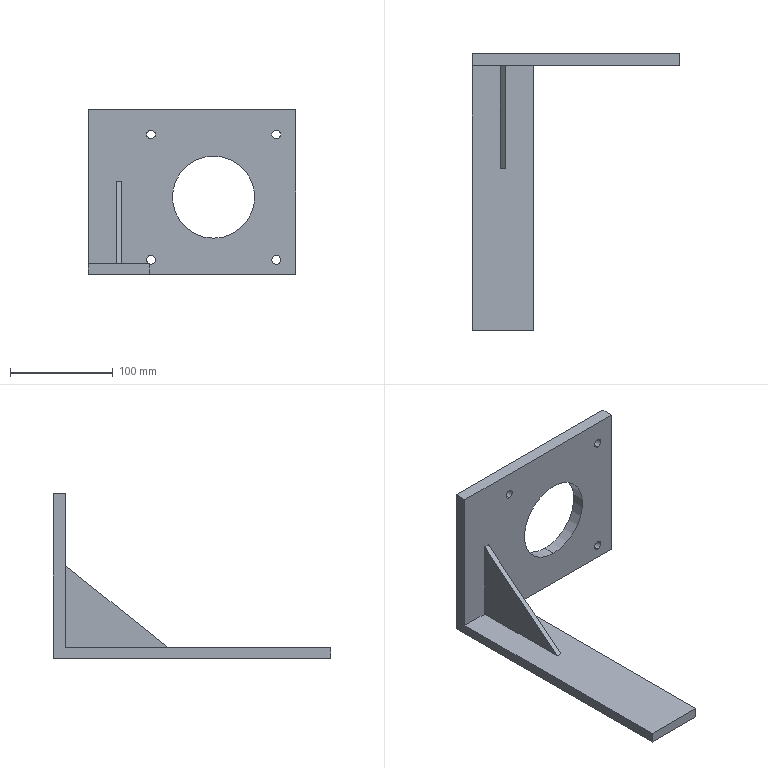Part | SolidWorks | features ICE 2, Extrusion 1, Gusset 1, HoleWzd 1 | 2 solids | 25 faces | box 202 x 270 x 160 mm | volume 499598 mm3 | plane 14 | cylinder 10 | cone 1 | commonest cylinder face diameters 8.5 x8 80 x2
STEP:
#1=CARTESIAN_POINT('',(30.,123.,9.869));
#2=VERTEX_POINT('',#1);
#3=CARTESIAN_POINT('',(31.,123.,9.75));
#4=VERTEX_POINT('',#3);
#5=CARTESIAN_POINT('',(31.,123.,14.));
#6=DIRECTION('',(0.,-1.,0.));
#7=DIRECTION('',(0.,0.,-1.));
#8=AXIS2_PLACEMENT_3D('',#5,#6,#7);
#9=CIRCLE('',#8,4.25);
#10=EDGE_CURVE('',#2,#4,#9,.T.);
#11=ORIENTED_EDGE('',*,*,#10,.T.);
#12=CARTESIAN_POINT('',(31.,135.,9.75));
#13=VERTEX_POINT('',#12);
#14=CARTESIAN_POINT('',(31.,135.,9.75));
#15=DIRECTION('',(0.,1.,0.));
#16=VECTOR('',#15,1000.);
#17=LINE('',#14,#16);
#18=EDGE_CURVE('',#4,#13,#17,.T.);
#19=ORIENTED_EDGE('',*,*,#18,.T.);
#20=CARTESIAN_POINT('',(31.,135.,18.25));
#21=VERTEX_POINT('',#20);
#22=CARTESIAN_POINT('',(31.,135.,14.));
#23=DIRECTION('',(0.,1.,0.));
#24=DIRECTION('',(0.,0.,1.));
#25=AXIS2_PLACEMENT_3D('',#22,#23,#24);
#26=CIRCLE('',#25,4.25);
#27=EDGE_CURVE('',#13,#21,#26,.T.);
#28=ORIENTED_EDGE('',*,*,#27,.T.);
#29=CARTESIAN_POINT('',(31.,123.,18.25));
#30=VERTEX_POINT('',#29);
#31=CARTESIAN_POINT('',(31.,135.,18.25));
#32=DIRECTION('',(0.,1.,0.));
#33=VECTOR('',#32,1000.);
#34=LINE('',#31,#33);
#35=EDGE_CURVE('',#30,#21,#34,.T.);
#36=ORIENTED_EDGE('',*,*,#35,.F.);
#37=CARTESIAN_POINT('',(29.564,123.,10.));
#38=VERTEX_POINT('',#37);
#39=CARTESIAN_POINT('',(31.,123.,14.));
#40=DIRECTION('',(0.,-1.,0.));
#41=DIRECTION('',(0.,0.,-1.));
#42=AXIS2_PLACEMENT_3D('',#39,#40,#41);
#43=CIRCLE('',#42,4.25);
#44=EDGE_CURVE('',#30,#38,#43,.T.);
#45=ORIENTED_EDGE('',*,*,#44,.T.);
#46=CARTESIAN_POINT('',(29.564,122.5,10.));
#47=VERTEX_POINT('',#46);
#48=CARTESIAN_POINT('',(29.564,135.,10.));
#49=DIRECTION('',(0.,1.,0.));
#50=VECTOR('',#49,1000.);
#51=LINE('',#48,#50);
#52=EDGE_CURVE('',#47,#38,#51,.T.);
#53=ORIENTED_EDGE('',*,*,#52,.F.);
#54=CARTESIAN_POINT('',(30.,122.5,9.869));
#55=VERTEX_POINT('',#54);
#56=CARTESIAN_POINT('',(31.,122.5,14.));
#57=DIRECTION('',(0.,1.,0.));
#58=DIRECTION('',(0.,0.,1.));
#59=AXIS2_PLACEMENT_3D('',#56,#57,#58);
#60=CIRCLE('',#59,4.25);
#61=EDGE_CURVE('',#55,#47,#60,.T.);
#62=ORIENTED_EDGE('',*,*,#61,.F.);
#63=CARTESIAN_POINT('',(30.,135.,9.869));
#64=DIRECTION('',(0.,-1.,0.));
#65=VECTOR('',#64,1000.);
#66=LINE('',#63,#65);
#67=EDGE_CURVE('',#2,#55,#66,.T.);
#68=ORIENTED_EDGE('',*,*,#67,.F.);
#69=EDGE_LOOP('',(#11,#19,#28,#36,#45,#53,#62,#68));
#70=FACE_OUTER_BOUND('',#69,.T.);
#71=CARTESIAN_POINT('',(31.,135.,14.));
#72=DIRECTION('',(0.,1.,0.));
#73=DIRECTION('',(0.,0.,1.));
#74=AXIS2_PLACEMENT_3D('',#71,#72,#73);
#75=CYLINDRICAL_SURFACE('',#74,4.25);
#76=ADVANCED_FACE('',(#70),#75,.F.);
#77=CARTESIAN_POINT('',(153.,123.,18.25));
#78=VERTEX_POINT('',#77);
#79=CARTESIAN_POINT('',(153.,123.,9.75));
#80=VERTEX_POINT('',#79);
#81=CARTESIAN_POINT('',(153.,123.,14.));
#82=DIRECTION('',(0.,-1.,0.));
#83=DIRECTION('',(0.,0.,-1.));
#84=AXIS2_PLACEMENT_3D('',#81,#82,#83);
#85=CIRCLE('',#84,4.25);
#86=EDGE_CURVE('',#78,#80,#85,.T.);
#87=ORIENTED_EDGE('',*,*,#86,.T.);
#88=CARTESIAN_POINT('',(153.,135.,9.75));
#89=VERTEX_POINT('',#88);
#90=CARTESIAN_POINT('',(153.,135.,9.75));
#91=DIRECTION('',(0.,1.,0.));
#92=VECTOR('',#91,1000.);
#93=LINE('',#90,#92);
#94=EDGE_CURVE('',#80,#89,#93,.T.);
#95=ORIENTED_EDGE('',*,*,#94,.T.);
#96=CARTESIAN_POINT('',(153.,135.,18.25));
#97=VERTEX_POINT('',#96);
#98=CARTESIAN_POINT('',(153.,135.,14.));
#99=DIRECTION('',(0.,1.,0.));
#100=DIRECTION('',(0.,0.,1.));
#101=AXIS2_PLACEMENT_3D('',#98,#99,#100);
#102=CIRCLE('',#101,4.25);
#103=EDGE_CURVE('',#89,#97,#102,.T.);
#104=ORIENTED_EDGE('',*,*,#103,.T.);
#105=CARTESIAN_POINT('',(153.,135.,18.25));
#106=DIRECTION('',(0.,1.,0.));
#107=VECTOR('',#106,1000.);
#108=LINE('',#105,#107);
#109=EDGE_CURVE('',#78,#97,#108,.T.);
#110=ORIENTED_EDGE('',*,*,#109,.F.);
#111=EDGE_LOOP('',(#87,#95,#104,#110));
#112=FACE_OUTER_BOUND('',#111,.T.);
#113=CARTESIAN_POINT('',(153.,135.,14.));
#114=DIRECTION('',(0.,1.,0.));
#115=DIRECTION('',(0.,0.,1.));
#116=AXIS2_PLACEMENT_3D('',#113,#114,#115);
#117=CYLINDRICAL_SURFACE('',#116,4.25);
#118=ADVANCED_FACE('',(#112),#117,.F.);
#119=CARTESIAN_POINT('',(153.,123.,140.25));
#120=VERTEX_POINT('',#119);
#121=CARTESIAN_POINT('',(153.,123.,131.75));
#122=VERTEX_POINT('',#121);
#123=CARTESIAN_POINT('',(153.,123.,136.));
#124=DIRECTION('',(0.,-1.,0.));
#125=DIRECTION('',(0.,0.,-1.));
#126=AXIS2_PLACEMENT_3D('',#123,#124,#125);
#127=CIRCLE('',#126,4.25);
#128=EDGE_CURVE('',#120,#122,#127,.T.);
#129=ORIENTED_EDGE('',*,*,#128,.T.);
#130=CARTESIAN_POINT('',(153.,135.,131.75));
#131=VERTEX_POINT('',#130);
#132=CARTESIAN_POINT('',(153.,135.,131.75));
#133=DIRECTION('',(0.,1.,0.));
#134=VECTOR('',#133,1000.);
#135=LINE('',#132,#134);
#136=EDGE_CURVE('',#122,#131,#135,.T.);
#137=ORIENTED_EDGE('',*,*,#136,.T.);
#138=CARTESIAN_POINT('',(153.,135.,140.25));
#139=VERTEX_POINT('',#138);
#140=CARTESIAN_POINT('',(153.,135.,136.));
#141=DIRECTION('',(0.,1.,0.));
#142=DIRECTION('',(0.,0.,1.));
#143=AXIS2_PLACEMENT_3D('',#140,#141,#142);
#144=CIRCLE('',#143,4.25);
#145=EDGE_CURVE('',#131,#139,#144,.T.);
#146=ORIENTED_EDGE('',*,*,#145,.T.);
#147=CARTESIAN_POINT('',(153.,135.,140.25));
#148=DIRECTION('',(0.,1.,0.));
#149=VECTOR('',#148,1000.);
#150=LINE('',#147,#149);
#151=EDGE_CURVE('',#120,#139,#150,.T.);
#152=ORIENTED_EDGE('',*,*,#151,.F.);
#153=EDGE_LOOP('',(#129,#137,#146,#152));
#154=FACE_OUTER_BOUND('',#153,.T.);
#155=CARTESIAN_POINT('',(153.,135.,136.));
#156=DIRECTION('',(0.,1.,0.));
#157=DIRECTION('',(0.,0.,1.));
#158=AXIS2_PLACEMENT_3D('',#155,#156,#157);
#159=CYLINDRICAL_SURFACE('',#158,4.25);
#160=ADVANCED_FACE('',(#154),#159,.F.);
#161=CARTESIAN_POINT('',(31.,123.,140.25));
#162=VERTEX_POINT('',#161);
#163=CARTESIAN_POINT('',(31.,123.,131.75));
#164=VERTEX_POINT('',#163);
#165=CARTESIAN_POINT('',(31.,123.,136.));
#166=DIRECTION('',(0.,-1.,0.));
#167=DIRECTION('',(0.,0.,-1.));
#168=AXIS2_PLACEMENT_3D('',#165,#166,#167);
#169=CIRCLE('',#168,4.25);
#170=EDGE_CURVE('',#162,#164,#169,.T.);
#171=ORIENTED_EDGE('',*,*,#170,.T.);
#172=CARTESIAN_POINT('',(31.,135.,131.75));
#173=VERTEX_POINT('',#172);
#174=CARTESIAN_POINT('',(31.,135.,131.75));
#175=DIRECTION('',(0.,1.,0.));
#176=VECTOR('',#175,1000.);
#177=LINE('',#174,#176);
#178=EDGE_CURVE('',#164,#173,#177,.T.);
#179=ORIENTED_EDGE('',*,*,#178,.T.);
#180=CARTESIAN_POINT('',(31.,135.,140.25));
#181=VERTEX_POINT('',#180);
#182=CARTESIAN_POINT('',(31.,135.,136.));
#183=DIRECTION('',(0.,1.,0.));
#184=DIRECTION('',(0.,0.,1.));
#185=AXIS2_PLACEMENT_3D('',#182,#183,#184);
#186=CIRCLE('',#185,4.25);
#187=EDGE_CURVE('',#173,#181,#186,.T.);
#188=ORIENTED_EDGE('',*,*,#187,.T.);
#189=CARTESIAN_POINT('',(31.,135.,140.25));
#190=DIRECTION('',(0.,1.,0.));
#191=VECTOR('',#190,1000.);
#192=LINE('',#189,#191);
#193=EDGE_CURVE('',#162,#181,#192,.T.);
#194=ORIENTED_EDGE('',*,*,#193,.F.);
#195=EDGE_LOOP('',(#171,#179,#188,#194));
#196=FACE_OUTER_BOUND('',#195,.T.);
#197=CARTESIAN_POINT('',(31.,135.,136.));
#198=DIRECTION('',(0.,1.,0.));
#199=DIRECTION('',(0.,0.,1.));
#200=AXIS2_PLACEMENT_3D('',#197,#198,#199);
#201=CYLINDRICAL_SURFACE('',#200,4.25);
#202=ADVANCED_FACE('',(#196),#201,.F.);
#203=CARTESIAN_POINT('',(92.,123.,115.));
#204=VERTEX_POINT('',#203);
#205=CARTESIAN_POINT('',(92.,123.,35.));
#206=VERTEX_POINT('',#205);
#207=CARTESIAN_POINT('',(92.,123.,75.));
#208=DIRECTION('',(0.,-1.,0.));
#209=DIRECTION('',(0.,0.,-1.));
#210=AXIS2_PLACEMENT_3D('',#207,#208,#209);
#211=CIRCLE('',#210,40.);
#212=EDGE_CURVE('',#204,#206,#211,.T.);
#213=ORIENTED_EDGE('',*,*,#212,.T.);
#214=CARTESIAN_POINT('',(92.,135.,35.));
#215=VERTEX_POINT('',#214);
#216=CARTESIAN_POINT('',(92.,-135.,35.));
#217=DIRECTION('',(0.,1.,0.));
#218=VECTOR('',#217,1000.);
#219=LINE('',#216,#218);
#220=EDGE_CURVE('',#206,#215,#219,.T.);
#221=ORIENTED_EDGE('',*,*,#220,.T.);
#222=CARTESIAN_POINT('',(92.,135.,115.));
#223=VERTEX_POINT('',#222);
#224=CARTESIAN_POINT('',(92.,135.,75.));
#225=DIRECTION('',(0.,1.,0.));
#226=DIRECTION('',(0.,0.,1.));
#227=AXIS2_PLACEMENT_3D('',#224,#225,#226);
#228=CIRCLE('',#227,40.);
#229=EDGE_CURVE('',#215,#223,#228,.T.);
#230=ORIENTED_EDGE('',*,*,#229,.T.);
#231=CARTESIAN_POINT('',(92.,-135.,115.));
#232=DIRECTION('',(0.,1.,0.));
#233=VECTOR('',#232,1000.);
#234=LINE('',#231,#233);
#235=EDGE_CURVE('',#204,#223,#234,.T.);
#236=ORIENTED_EDGE('',*,*,#235,.F.);
#237=EDGE_LOOP('',(#213,#221,#230,#236));
#238=FACE_OUTER_BOUND('',#237,.T.);
#239=CARTESIAN_POINT('',(92.,-135.,75.));
#240=DIRECTION('',(0.,1.,0.));
#241=DIRECTION('',(0.,0.,1.));
#242=AXIS2_PLACEMENT_3D('',#239,#240,#241);
#243=CYLINDRICAL_SURFACE('',#242,40.);
#244=ADVANCED_FACE('',(#238),#243,.F.);
#245=CARTESIAN_POINT('',(30.,123.,0.));
#246=VERTEX_POINT('',#245);
#247=CARTESIAN_POINT('',(30.,123.,10.));
#248=DIRECTION('',(0.,0.,1.));
#249=VECTOR('',#248,1000.);
#250=LINE('',#247,#249);
#251=EDGE_CURVE('',#246,#2,#250,.T.);
#252=ORIENTED_EDGE('',*,*,#251,.T.);
#253=ORIENTED_EDGE('',*,*,#67,.T.);
#254=CARTESIAN_POINT('',(30.,122.424,10.));
#255=VERTEX_POINT('',#254);
#256=CARTESIAN_POINT('',(30.,122.5,9.869));
#257=CARTESIAN_POINT('',(30.,122.475,9.913));
#258=CARTESIAN_POINT('',(30.,122.449,9.956));
#259=CARTESIAN_POINT('',(30.,122.424,10.));
#260=B_SPLINE_CURVE_WITH_KNOTS('',3,(#256,#257,#258,#259),.UNSPECIFIED.,.F.,.F.,(4,4),(0.004492,0.004643),.UNSPECIFIED.);
#261=EDGE_CURVE('',#55,#255,#260,.T.);
#262=ORIENTED_EDGE('',*,*,#261,.T.);
#263=CARTESIAN_POINT('',(30.,-135.,10.));
#264=VERTEX_POINT('',#263);
#265=CARTESIAN_POINT('',(30.,-135.,10.));
#266=DIRECTION('',(0.,1.,0.));
#267=VECTOR('',#266,1000.);
#268=LINE('',#265,#267);
#269=EDGE_CURVE('',#264,#255,#268,.T.);
#270=ORIENTED_EDGE('',*,*,#269,.F.);
#271=CARTESIAN_POINT('',(30.,-135.,0.));
#272=VERTEX_POINT('',#271);
#273=CARTESIAN_POINT('',(30.,-135.,10.));
#274=DIRECTION('',(0.,0.,-1.));
#275=VECTOR('',#274,1000.);
#276=LINE('',#273,#275);
#277=EDGE_CURVE('',#264,#272,#276,.T.);
#278=ORIENTED_EDGE('',*,*,#277,.T.);
#279=CARTESIAN_POINT('',(30.,-135.,0.));
#280=DIRECTION('',(0.,1.,0.));
#281=VECTOR('',#280,1000.);
#282=LINE('',#279,#281);
#283=EDGE_CURVE('',#272,#246,#282,.T.);
#284=ORIENTED_EDGE('',*,*,#283,.T.);
#285=EDGE_LOOP('',(#252,#253,#262,#270,#278,#284));
#286=FACE_OUTER_BOUND('',#285,.T.);
#287=CARTESIAN_POINT('',(30.,-135.,10.));
#288=DIRECTION('',(-1.,0.,0.));
#289=DIRECTION('',(0.,0.,1.));
#290=AXIS2_PLACEMENT_3D('',#287,#288,#289);
#291=PLANE('',#290);
#292=ADVANCED_FACE('',(#286),#291,.F.);
#293=CARTESIAN_POINT('',(31.,135.,14.));
#294=DIRECTION('',(0.,1.,0.));
#295=DIRECTION('',(0.,0.,1.));
#296=AXIS2_PLACEMENT_3D('',#293,#294,#295);
#297=CIRCLE('',#296,4.25);
#298=EDGE_CURVE('',#21,#13,#297,.T.);
#299=ORIENTED_EDGE('',*,*,#298,.F.);
#300=ORIENTED_EDGE('',*,*,#27,.F.);
#301=EDGE_LOOP('',(#299,#300));
#302=FACE_BOUND('',#301,.T.);
#303=CARTESIAN_POINT('',(153.,135.,14.));
#304=DIRECTION('',(0.,1.,0.));
#305=DIRECTION('',(0.,0.,1.));
#306=AXIS2_PLACEMENT_3D('',#303,#304,#305);
#307=CIRCLE('',#306,4.25);
#308=EDGE_CURVE('',#97,#89,#307,.T.);
#309=ORIENTED_EDGE('',*,*,#308,.F.);
#310=ORIENTED_EDGE('',*,*,#103,.F.);
#311=EDGE_LOOP('',(#309,#310));
#312=FACE_BOUND('',#311,.T.);
#313=CARTESIAN_POINT('',(153.,135.,136.));
#314=DIRECTION('',(0.,1.,0.));
#315=DIRECTION('',(0.,0.,1.));
#316=AXIS2_PLACEMENT_3D('',#313,#314,#315);
#317=CIRCLE('',#316,4.25);
#318=EDGE_CURVE('',#139,#131,#317,.T.);
#319=ORIENTED_EDGE('',*,*,#318,.F.);
#320=ORIENTED_EDGE('',*,*,#145,.F.);
#321=EDGE_LOOP('',(#319,#320));
#322=FACE_BOUND('',#321,.T.);
#323=CARTESIAN_POINT('',(31.,135.,136.));
#324=DIRECTION('',(0.,1.,0.));
#325=DIRECTION('',(0.,0.,1.));
#326=AXIS2_PLACEMENT_3D('',#323,#324,#325);
#327=CIRCLE('',#326,4.25);
#328=EDGE_CURVE('',#181,#173,#327,.T.);
#329=ORIENTED_EDGE('',*,*,#328,.F.);
#330=ORIENTED_EDGE('',*,*,#187,.F.);
#331=EDGE_LOOP('',(#329,#330));
#332=FACE_BOUND('',#331,.T.);
#333=CARTESIAN_POINT('',(92.,135.,75.));
#334=DIRECTION('',(0.,1.,0.));
#335=DIRECTION('',(0.,0.,1.));
#336=AXIS2_PLACEMENT_3D('',#333,#334,#335);
#337=CIRCLE('',#336,40.);
#338=EDGE_CURVE('',#223,#215,#337,.T.);
#339=ORIENTED_EDGE('',*,*,#338,.F.);
#340=ORIENTED_EDGE('',*,*,#229,.F.);
#341=EDGE_LOOP('',(#339,#340));
#342=FACE_BOUND('',#341,.T.);
#343=CARTESIAN_POINT('',(172.,135.,0.));
#344=VERTEX_POINT('',#343);
#345=CARTESIAN_POINT('',(172.,135.,160.));
#346=VERTEX_POINT('',#345);
#347=CARTESIAN_POINT('',(172.,135.,0.));
#348=DIRECTION('',(0.,0.,1.));
#349=VECTOR('',#348,1000.);
#350=LINE('',#347,#349);
#351=EDGE_CURVE('',#344,#346,#350,.T.);
#352=ORIENTED_EDGE('',*,*,#351,.F.);
#353=CARTESIAN_POINT('',(-30.,135.,0.));
#354=VERTEX_POINT('',#353);
#355=CARTESIAN_POINT('',(-30.,135.,0.));
#356=DIRECTION('',(-1.,0.,0.));
#357=VECTOR('',#356,1000.);
#358=LINE('',#355,#357);
#359=EDGE_CURVE('',#344,#354,#358,.T.);
#360=ORIENTED_EDGE('',*,*,#359,.T.);
#361=CARTESIAN_POINT('',(-30.,135.,160.));
#362=VERTEX_POINT('',#361);
#363=CARTESIAN_POINT('',(-30.,135.,10.));
#364=DIRECTION('',(0.,0.,-1.));
#365=VECTOR('',#364,1000.);
#366=LINE('',#363,#365);
#367=EDGE_CURVE('',#362,#354,#366,.T.);
#368=ORIENTED_EDGE('',*,*,#367,.F.);
#369=CARTESIAN_POINT('',(-30.,135.,160.));
#370=DIRECTION('',(-1.,0.,0.));
#371=VECTOR('',#370,1000.);
#372=LINE('',#369,#371);
#373=EDGE_CURVE('',#346,#362,#372,.T.);
#374=ORIENTED_EDGE('',*,*,#373,.F.);
#375=EDGE_LOOP('',(#352,#360,#368,#374));
#376=FACE_OUTER_BOUND('',#375,.T.);
#377=CARTESIAN_POINT('',(-30.,135.,10.));
#378=DIRECTION('',(0.,-1.,0.));
#379=DIRECTION('',(0.,0.,-1.));
#380=AXIS2_PLACEMENT_3D('',#377,#378,#379);
#381=PLANE('',#380);
#382=ADVANCED_FACE('',(#302,#312,#322,#332,#342,#376),#381,.F.);
#383=CARTESIAN_POINT('',(-30.,123.,10.));
#384=VERTEX_POINT('',#383);
#385=CARTESIAN_POINT('',(-30.,-135.,10.));
#386=VERTEX_POINT('',#385);
#387=CARTESIAN_POINT('',(-30.,-135.,10.));
#388=DIRECTION('',(0.,-1.,0.));
#389=VECTOR('',#388,1000.);
#390=LINE('',#387,#389);
#391=EDGE_CURVE('',#384,#386,#390,.T.);
#392=ORIENTED_EDGE('',*,*,#391,.F.);
#393=CARTESIAN_POINT('',(-30.,123.,160.));
#394=VERTEX_POINT('',#393);
#395=CARTESIAN_POINT('',(-30.,123.,0.));
#396=DIRECTION('',(0.,0.,1.));
#397=VECTOR('',#396,1000.);
#398=LINE('',#395,#397);
#399=EDGE_CURVE('',#384,#394,#398,.T.);
#400=ORIENTED_EDGE('',*,*,#399,.T.);
#401=CARTESIAN_POINT('',(-30.,135.,160.));
#402=DIRECTION('',(0.,-1.,0.));
#403=VECTOR('',#402,1000.);
#404=LINE('',#401,#403);
#405=EDGE_CURVE('',#362,#394,#404,.T.);
#406=ORIENTED_EDGE('',*,*,#405,.F.);
#407=ORIENTED_EDGE('',*,*,#367,.T.);
#408=CARTESIAN_POINT('',(-30.,-135.,0.));
#409=VERTEX_POINT('',#408);
#410=CARTESIAN_POINT('',(-30.,-135.,0.));
#411=DIRECTION('',(0.,-1.,0.));
#412=VECTOR('',#411,1000.);
#413=LINE('',#410,#412);
#414=EDGE_CURVE('',#354,#409,#413,.T.);
#415=ORIENTED_EDGE('',*,*,#414,.T.);
#416=CARTESIAN_POINT('',(-30.,-135.,10.));
#417=DIRECTION('',(0.,0.,-1.));
#418=VECTOR('',#417,1000.);
#419=LINE('',#416,#418);
#420=EDGE_CURVE('',#386,#409,#419,.T.);
#421=ORIENTED_EDGE('',*,*,#420,.F.);
#422=EDGE_LOOP('',(#392,#400,#406,#407,#415,#421));
#423=FACE_OUTER_BOUND('',#422,.T.);
#424=CARTESIAN_POINT('',(-30.,-135.,10.));
#425=DIRECTION('',(1.,0.,0.));
#426=DIRECTION('',(0.,0.,-1.));
#427=AXIS2_PLACEMENT_3D('',#424,#425,#426);
#428=PLANE('',#427);
#429=ADVANCED_FACE('',(#423),#428,.F.);
#430=CARTESIAN_POINT('',(-30.,-135.,0.));
#431=DIRECTION('',(1.,0.,0.));
#432=VECTOR('',#431,1000.);
#433=LINE('',#430,#432);
#434=EDGE_CURVE('',#409,#272,#433,.T.);
#435=ORIENTED_EDGE('',*,*,#434,.T.);
#436=ORIENTED_EDGE('',*,*,#277,.F.);
#437=CARTESIAN_POINT('',(-30.,-135.,10.));
#438=DIRECTION('',(1.,0.,0.));
#439=VECTOR('',#438,1000.);
#440=LINE('',#437,#439);
#441=EDGE_CURVE('',#386,#264,#440,.T.);
#442=ORIENTED_EDGE('',*,*,#441,.F.);
#443=ORIENTED_EDGE('',*,*,#420,.T.);
#444=EDGE_LOOP('',(#435,#436,#442,#443));
#445=FACE_OUTER_BOUND('',#444,.T.);
#446=CARTESIAN_POINT('',(-30.,-135.,10.));
#447=DIRECTION('',(0.,1.,0.));
#448=DIRECTION('',(0.,0.,1.));
#449=AXIS2_PLACEMENT_3D('',#446,#447,#448);
#450=PLANE('',#449);
#451=ADVANCED_FACE('',(#445),#450,.F.);
#452=CARTESIAN_POINT('',(30.,122.424,10.));
#453=CARTESIAN_POINT('',(29.853,122.445,10.));
#454=CARTESIAN_POINT('',(29.708,122.471,10.));
#455=CARTESIAN_POINT('',(29.564,122.5,10.));
#456=B_SPLINE_CURVE_WITH_KNOTS('',3,(#452,#453,#454,#455),.UNSPECIFIED.,.F.,.F.,(4,4),(0.002482,0.002922),.UNSPECIFIED.);
#457=EDGE_CURVE('',#255,#47,#456,.T.);
#458=ORIENTED_EDGE('',*,*,#457,.T.);
#459=ORIENTED_EDGE('',*,*,#52,.T.);
#460=CARTESIAN_POINT('',(0.,123.,10.));
#461=DIRECTION('',(-1.,0.,0.));
#462=VECTOR('',#461,1000.);
#463=LINE('',#460,#462);
#464=EDGE_CURVE('',#38,#384,#463,.T.);
#465=ORIENTED_EDGE('',*,*,#464,.T.);
#466=ORIENTED_EDGE('',*,*,#391,.T.);
#467=ORIENTED_EDGE('',*,*,#441,.T.);
#468=ORIENTED_EDGE('',*,*,#269,.T.);
#469=EDGE_LOOP('',(#458,#459,#465,#466,#467,#468));
#470=FACE_OUTER_BOUND('',#469,.T.);
#471=CARTESIAN_POINT('',(0.,0.,10.));
#472=DIRECTION('',(0.,0.,-1.));
#473=DIRECTION('',(-1.,0.,0.));
#474=AXIS2_PLACEMENT_3D('',#471,#472,#473);
#475=PLANE('',#474);
#476=ADVANCED_FACE('',(#470),#475,.F.);
#477=ORIENTED_EDGE('',*,*,#434,.F.);
#478=ORIENTED_EDGE('',*,*,#414,.F.);
#479=ORIENTED_EDGE('',*,*,#359,.F.);
#480=CARTESIAN_POINT('',(172.,123.,0.));
#481=VERTEX_POINT('',#480);
#482=CARTESIAN_POINT('',(172.,135.,0.));
#483=DIRECTION('',(0.,1.,0.));
#484=VECTOR('',#483,1000.);
#485=LINE('',#482,#484);
#486=EDGE_CURVE('',#481,#344,#485,.T.);
#487=ORIENTED_EDGE('',*,*,#486,.F.);
#488=CARTESIAN_POINT('',(-30.,123.,0.));
#489=DIRECTION('',(1.,0.,0.));
#490=VECTOR('',#489,1000.);
#491=LINE('',#488,#490);
#492=EDGE_CURVE('',#246,#481,#491,.T.);
#493=ORIENTED_EDGE('',*,*,#492,.F.);
#494=ORIENTED_EDGE('',*,*,#283,.F.);
#495=EDGE_LOOP('',(#477,#478,#479,#487,#493,#494));
#496=FACE_OUTER_BOUND('',#495,.T.);
#497=CARTESIAN_POINT('',(0.,0.,0.));
#498=DIRECTION('',(0.,0.,-1.));
#499=DIRECTION('',(-1.,0.,0.));
#500=AXIS2_PLACEMENT_3D('',#497,#498,#499);
#501=PLANE('',#500);
#502=ADVANCED_FACE('',(#496),#501,.T.);
#503=ORIENTED_EDGE('',*,*,#10,.F.);
#504=ORIENTED_EDGE('',*,*,#251,.F.);
#505=ORIENTED_EDGE('',*,*,#492,.T.);
#506=CARTESIAN_POINT('',(172.,123.,160.));
#507=VERTEX_POINT('',#506);
#508=CARTESIAN_POINT('',(172.,123.,0.));
#509=DIRECTION('',(0.,0.,1.));
#510=VECTOR('',#509,1000.);
#511=LINE('',#508,#510);
#512=EDGE_CURVE('',#481,#507,#511,.T.);
#513=ORIENTED_EDGE('',*,*,#512,.T.);
#514=CARTESIAN_POINT('',(-30.,123.,160.));
#515=DIRECTION('',(1.,0.,0.));
#516=VECTOR('',#515,1000.);
#517=LINE('',#514,#516);
#518=EDGE_CURVE('',#394,#507,#517,.T.);
#519=ORIENTED_EDGE('',*,*,#518,.F.);
#520=ORIENTED_EDGE('',*,*,#399,.F.);
#521=ORIENTED_EDGE('',*,*,#464,.F.);
#522=ORIENTED_EDGE('',*,*,#44,.F.);
#523=CARTESIAN_POINT('',(31.,123.,14.));
#524=DIRECTION('',(0.,-1.,0.));
#525=DIRECTION('',(0.,0.,-1.));
#526=AXIS2_PLACEMENT_3D('',#523,#524,#525);
#527=CIRCLE('',#526,4.25);
#528=EDGE_CURVE('',#4,#30,#527,.T.);
#529=ORIENTED_EDGE('',*,*,#528,.F.);
#530=EDGE_LOOP('',(#503,#504,#505,#513,#519,#520,#521,#522,#529));
#531=FACE_OUTER_BOUND('',#530,.T.);
#532=ORIENTED_EDGE('',*,*,#86,.F.);
#533=CARTESIAN_POINT('',(153.,123.,14.));
#534=DIRECTION('',(0.,-1.,0.));
#535=DIRECTION('',(0.,0.,-1.));
#536=AXIS2_PLACEMENT_3D('',#533,#534,#535);
#537=CIRCLE('',#536,4.25);
#538=EDGE_CURVE('',#80,#78,#537,.T.);
#539=ORIENTED_EDGE('',*,*,#538,.F.);
#540=EDGE_LOOP('',(#532,#539));
#541=FACE_BOUND('',#540,.T.);
#542=ORIENTED_EDGE('',*,*,#128,.F.);
#543=CARTESIAN_POINT('',(153.,123.,136.));
#544=DIRECTION('',(0.,-1.,0.));
#545=DIRECTION('',(0.,0.,-1.));
#546=AXIS2_PLACEMENT_3D('',#543,#544,#545);
#547=CIRCLE('',#546,4.25);
#548=EDGE_CURVE('',#122,#120,#547,.T.);
#549=ORIENTED_EDGE('',*,*,#548,.F.);
#550=EDGE_LOOP('',(#542,#549));
#551=FACE_BOUND('',#550,.T.);
#552=ORIENTED_EDGE('',*,*,#170,.F.);
#553=CARTESIAN_POINT('',(31.,123.,136.));
#554=DIRECTION('',(0.,-1.,0.));
#555=DIRECTION('',(0.,0.,-1.));
#556=AXIS2_PLACEMENT_3D('',#553,#554,#555);
#557=CIRCLE('',#556,4.25);
#558=EDGE_CURVE('',#164,#162,#557,.T.);
#559=ORIENTED_EDGE('',*,*,#558,.F.);
#560=EDGE_LOOP('',(#552,#559));
#561=FACE_BOUND('',#560,.T.);
#562=ORIENTED_EDGE('',*,*,#212,.F.);
#563=CARTESIAN_POINT('',(92.,123.,75.));
#564=DIRECTION('',(0.,-1.,0.));
#565=DIRECTION('',(0.,0.,-1.));
#566=AXIS2_PLACEMENT_3D('',#563,#564,#565);
#567=CIRCLE('',#566,40.);
#568=EDGE_CURVE('',#206,#204,#567,.T.);
#569=ORIENTED_EDGE('',*,*,#568,.F.);
#570=EDGE_LOOP('',(#562,#569));
#571=FACE_BOUND('',#570,.T.);
#572=CARTESIAN_POINT('',(-30.,123.,0.));
#573=DIRECTION('',(0.,-1.,0.));
#574=DIRECTION('',(0.,0.,-1.));
#575=AXIS2_PLACEMENT_3D('',#572,#573,#574);
#576=PLANE('',#575);
#577=ADVANCED_FACE('',(#531,#541,#551,#561,#571),#576,.T.);
#578=ORIENTED_EDGE('',*,*,#351,.T.);
#579=CARTESIAN_POINT('',(172.,135.,160.));
#580=DIRECTION('',(0.,1.,0.));
#581=VECTOR('',#580,1000.);
#582=LINE('',#579,#581);
#583=EDGE_CURVE('',#507,#346,#582,.T.);
#584=ORIENTED_EDGE('',*,*,#583,.F.);
#585=ORIENTED_EDGE('',*,*,#512,.F.);
#586=ORIENTED_EDGE('',*,*,#486,.T.);
#587=EDGE_LOOP('',(#578,#584,#585,#586));
#588=FACE_OUTER_BOUND('',#587,.T.);
#589=CARTESIAN_POINT('',(172.,135.,0.));
#590=DIRECTION('',(1.,0.,0.));
#591=DIRECTION('',(0.,0.,-1.));
#592=AXIS2_PLACEMENT_3D('',#589,#590,#591);
#593=PLANE('',#592);
#594=ADVANCED_FACE('',(#588),#593,.T.);
#595=ORIENTED_EDGE('',*,*,#405,.T.);
#596=ORIENTED_EDGE('',*,*,#518,.T.);
#597=ORIENTED_EDGE('',*,*,#583,.T.);
#598=ORIENTED_EDGE('',*,*,#373,.T.);
#599=EDGE_LOOP('',(#595,#596,#597,#598));
#600=FACE_OUTER_BOUND('',#599,.T.);
#601=CARTESIAN_POINT('',(0.,0.,160.));
#602=DIRECTION('',(0.,0.,1.));
#603=DIRECTION('',(1.,0.,0.));
#604=AXIS2_PLACEMENT_3D('',#601,#602,#603);
#605=PLANE('',#604);
#606=ADVANCED_FACE('',(#600),#605,.T.);
#607=ORIENTED_EDGE('',*,*,#220,.F.);
#608=ORIENTED_EDGE('',*,*,#568,.T.);
#609=ORIENTED_EDGE('',*,*,#235,.T.);
#610=ORIENTED_EDGE('',*,*,#338,.T.);
#611=EDGE_LOOP('',(#607,#608,#609,#610));
#612=FACE_OUTER_BOUND('',#611,.T.);
#613=CARTESIAN_POINT('',(92.,-135.,75.));
#614=DIRECTION('',(0.,1.,0.));
#615=DIRECTION('',(0.,0.,1.));
#616=AXIS2_PLACEMENT_3D('',#613,#614,#615);
#617=CYLINDRICAL_SURFACE('',#616,40.);
#618=ADVANCED_FACE('',(#612),#617,.F.);
#619=ORIENTED_EDGE('',*,*,#178,.F.);
#620=ORIENTED_EDGE('',*,*,#558,.T.);
#621=ORIENTED_EDGE('',*,*,#193,.T.);
#622=ORIENTED_EDGE('',*,*,#328,.T.);
#623=EDGE_LOOP('',(#619,#620,#621,#622));
#624=FACE_OUTER_BOUND('',#623,.T.);
#625=CARTESIAN_POINT('',(31.,135.,136.));
#626=DIRECTION('',(0.,1.,0.));
#627=DIRECTION('',(0.,0.,1.));
#628=AXIS2_PLACEMENT_3D('',#625,#626,#627);
#629=CYLINDRICAL_SURFACE('',#628,4.25);
#630=ADVANCED_FACE('',(#624),#629,.F.);
#631=ORIENTED_EDGE('',*,*,#136,.F.);
#632=ORIENTED_EDGE('',*,*,#548,.T.);
#633=ORIENTED_EDGE('',*,*,#151,.T.);
#634=ORIENTED_EDGE('',*,*,#318,.T.);
#635=EDGE_LOOP('',(#631,#632,#633,#634));
#636=FACE_OUTER_BOUND('',#635,.T.);
#637=CARTESIAN_POINT('',(153.,135.,136.));
#638=DIRECTION('',(0.,1.,0.));
#639=DIRECTION('',(0.,0.,1.));
#640=AXIS2_PLACEMENT_3D('',#637,#638,#639);
#641=CYLINDRICAL_SURFACE('',#640,4.25);
#642=ADVANCED_FACE('',(#636),#641,.F.);
#643=ORIENTED_EDGE('',*,*,#94,.F.);
#644=ORIENTED_EDGE('',*,*,#538,.T.);
#645=ORIENTED_EDGE('',*,*,#109,.T.);
#646=ORIENTED_EDGE('',*,*,#308,.T.);
#647=EDGE_LOOP('',(#643,#644,#645,#646));
#648=FACE_OUTER_BOUND('',#647,.T.);
#649=CARTESIAN_POINT('',(153.,135.,14.));
#650=DIRECTION('',(0.,1.,0.));
#651=DIRECTION('',(0.,0.,1.));
#652=AXIS2_PLACEMENT_3D('',#649,#650,#651);
#653=CYLINDRICAL_SURFACE('',#652,4.25);
#654=ADVANCED_FACE('',(#648),#653,.F.);
#655=ORIENTED_EDGE('',*,*,#18,.F.);
#656=ORIENTED_EDGE('',*,*,#528,.T.);
#657=ORIENTED_EDGE('',*,*,#35,.T.);
#658=ORIENTED_EDGE('',*,*,#298,.T.);
#659=EDGE_LOOP('',(#655,#656,#657,#658));
#660=FACE_OUTER_BOUND('',#659,.T.);
#661=CARTESIAN_POINT('',(31.,135.,14.));
#662=DIRECTION('',(0.,1.,0.));
#663=DIRECTION('',(0.,0.,1.));
#664=AXIS2_PLACEMENT_3D('',#661,#662,#663);
#665=CYLINDRICAL_SURFACE('',#664,4.25);
#666=ADVANCED_FACE('',(#660),#665,.F.);
#667=ORIENTED_EDGE('',*,*,#61,.T.);
#668=ORIENTED_EDGE('',*,*,#457,.F.);
#669=ORIENTED_EDGE('',*,*,#261,.F.);
#670=EDGE_LOOP('',(#667,#668,#669));
#671=FACE_OUTER_BOUND('',#670,.T.);
#672=CARTESIAN_POINT('',(31.,122.5,14.));
#673=DIRECTION('',(0.,1.,0.));
#674=DIRECTION('',(0.,0.,1.));
#675=AXIS2_PLACEMENT_3D('',#672,#673,#674);
#676=CONICAL_SURFACE('',#675,4.25,1.03);
#677=ADVANCED_FACE('',(#671),#676,.F.);
#678=CLOSED_SHELL('',(#76,#118,#160,#202,#244,#292,#382,#429,#451,#476,#502,#577,#594,#606,#618,#630,#642,#654,#666,#677));
#679=MANIFOLD_SOLID_BREP('',#678);
#680=CARTESIAN_POINT('',(-2.718,123.,90.));
#681=VERTEX_POINT('',#680);
#682=CARTESIAN_POINT('',(-2.718,23.,10.));
#683=VERTEX_POINT('',#682);
#684=CARTESIAN_POINT('',(-2.718,123.,90.));
#685=DIRECTION('',(0.,-0.7809,-0.6247));
#686=VECTOR('',#685,1000.);
#687=LINE('',#684,#686);
#688=EDGE_CURVE('',#681,#683,#687,.T.);
#689=ORIENTED_EDGE('',*,*,#688,.T.);
#690=CARTESIAN_POINT('',(2.282,23.,10.));
#691=VERTEX_POINT('',#690);
#692=CARTESIAN_POINT('',(2.282,23.,10.));
#693=DIRECTION('',(-1.,0.,0.));
#694=VECTOR('',#693,1000.);
#695=LINE('',#692,#694);
#696=EDGE_CURVE('',#691,#683,#695,.T.);
#697=ORIENTED_EDGE('',*,*,#696,.F.);
#698=CARTESIAN_POINT('',(2.282,123.,90.));
#699=VERTEX_POINT('',#698);
#700=CARTESIAN_POINT('',(2.282,123.,90.));
#701=DIRECTION('',(0.,-0.7809,-0.6247));
#702=VECTOR('',#701,1000.);
#703=LINE('',#700,#702);
#704=EDGE_CURVE('',#699,#691,#703,.T.);
#705=ORIENTED_EDGE('',*,*,#704,.F.);
#706=CARTESIAN_POINT('',(2.282,123.,90.));
#707=DIRECTION('',(-1.,0.,0.));
#708=VECTOR('',#707,1000.);
#709=LINE('',#706,#708);
#710=EDGE_CURVE('',#699,#681,#709,.T.);
#711=ORIENTED_EDGE('',*,*,#710,.T.);
#712=EDGE_LOOP('',(#689,#697,#705,#711));
#713=FACE_OUTER_BOUND('',#712,.T.);
#714=CARTESIAN_POINT('',(2.282,123.,90.));
#715=DIRECTION('',(0.,0.6247,-0.7809));
#716=DIRECTION('',(0.,0.7809,0.6247));
#717=AXIS2_PLACEMENT_3D('',#714,#715,#716);
#718=PLANE('',#717);
#719=ADVANCED_FACE('',(#713),#718,.F.);
#720=CARTESIAN_POINT('',(-2.718,123.,10.));
#721=VERTEX_POINT('',#720);
#722=CARTESIAN_POINT('',(-2.718,123.,10.));
#723=DIRECTION('',(0.,1.,0.));
#724=VECTOR('',#723,1000.);
#725=LINE('',#722,#724);
#726=EDGE_CURVE('',#683,#721,#725,.T.);
#727=ORIENTED_EDGE('',*,*,#726,.T.);
#728=CARTESIAN_POINT('',(2.282,123.,10.));
#729=VERTEX_POINT('',#728);
#730=CARTESIAN_POINT('',(2.282,123.,10.));
#731=DIRECTION('',(-1.,0.,0.));
#732=VECTOR('',#731,1000.);
#733=LINE('',#730,#732);
#734=EDGE_CURVE('',#729,#721,#733,.T.);
#735=ORIENTED_EDGE('',*,*,#734,.F.);
#736=CARTESIAN_POINT('',(2.282,123.,10.));
#737=DIRECTION('',(0.,1.,0.));
#738=VECTOR('',#737,1000.);
#739=LINE('',#736,#738);
#740=EDGE_CURVE('',#691,#729,#739,.T.);
#741=ORIENTED_EDGE('',*,*,#740,.F.);
#742=ORIENTED_EDGE('',*,*,#696,.T.);
#743=EDGE_LOOP('',(#727,#735,#741,#742));
#744=FACE_OUTER_BOUND('',#743,.T.);
#745=CARTESIAN_POINT('',(2.282,123.,10.));
#746=DIRECTION('',(0.,0.,1.));
#747=DIRECTION('',(1.,0.,0.));
#748=AXIS2_PLACEMENT_3D('',#745,#746,#747);
#749=PLANE('',#748);
#750=ADVANCED_FACE('',(#744),#749,.F.);
#751=CARTESIAN_POINT('',(-2.718,123.,10.));
#752=DIRECTION('',(0.,0.,1.));
#753=VECTOR('',#752,1000.);
#754=LINE('',#751,#753);
#755=EDGE_CURVE('',#721,#681,#754,.T.);
#756=ORIENTED_EDGE('',*,*,#755,.T.);
#757=ORIENTED_EDGE('',*,*,#710,.F.);
#758=CARTESIAN_POINT('',(2.282,123.,10.));
#759=DIRECTION('',(0.,0.,1.));
#760=VECTOR('',#759,1000.);
#761=LINE('',#758,#760);
#762=EDGE_CURVE('',#729,#699,#761,.T.);
#763=ORIENTED_EDGE('',*,*,#762,.F.);
#764=ORIENTED_EDGE('',*,*,#734,.T.);
#765=EDGE_LOOP('',(#756,#757,#763,#764));
#766=FACE_OUTER_BOUND('',#765,.T.);
#767=CARTESIAN_POINT('',(2.282,123.,10.));
#768=DIRECTION('',(0.,-1.,0.));
#769=DIRECTION('',(1.,0.,0.));
#770=AXIS2_PLACEMENT_3D('',#767,#768,#769);
#771=PLANE('',#770);
#772=ADVANCED_FACE('',(#766),#771,.F.);
#773=ORIENTED_EDGE('',*,*,#704,.T.);
#774=ORIENTED_EDGE('',*,*,#740,.T.);
#775=ORIENTED_EDGE('',*,*,#762,.T.);
#776=EDGE_LOOP('',(#773,#774,#775));
#777=FACE_OUTER_BOUND('',#776,.T.);
#778=CARTESIAN_POINT('',(2.282,0.,0.));
#779=DIRECTION('',(-1.,0.,0.));
#780=DIRECTION('',(0.,-1.,0.));
#781=AXIS2_PLACEMENT_3D('',#778,#779,#780);
#782=PLANE('',#781);
#783=ADVANCED_FACE('',(#777),#782,.F.);
#784=ORIENTED_EDGE('',*,*,#688,.F.);
#785=ORIENTED_EDGE('',*,*,#755,.F.);
#786=ORIENTED_EDGE('',*,*,#726,.F.);
#787=EDGE_LOOP('',(#784,#785,#786));
#788=FACE_OUTER_BOUND('',#787,.T.);
#789=CARTESIAN_POINT('',(-2.718,0.,0.));
#790=DIRECTION('',(-1.,0.,0.));
#791=DIRECTION('',(0.,-1.,0.));
#792=AXIS2_PLACEMENT_3D('',#789,#790,#791);
#793=PLANE('',#792);
#794=ADVANCED_FACE('',(#788),#793,.T.);
#795=CLOSED_SHELL('',(#719,#750,#772,#783,#794));
#796=MANIFOLD_SOLID_BREP('',#795);
#797=CARTESIAN_POINT('',(0.,0.,0.));
#798=DIRECTION('',(0.,0.,1.));
#799=DIRECTION('',(1.,0.,0.));
#800=AXIS2_PLACEMENT_3D('',#797,#798,#799);
#801=(LENGTH_UNIT()NAMED_UNIT(*)SI_UNIT(.MILLI.,.METRE.));
#802=UNCERTAINTY_MEASURE_WITH_UNIT(LENGTH_MEASURE(0.00001),#801,'','');
#803=(NAMED_UNIT(*)PLANE_ANGLE_UNIT()SI_UNIT($,.RADIAN.));
#804=(NAMED_UNIT(*)SI_UNIT($,.STERADIAN.)SOLID_ANGLE_UNIT());
#805=(GEOMETRIC_REPRESENTATION_CONTEXT(3)GLOBAL_UNCERTAINTY_ASSIGNED_CONTEXT((#802))GLOBAL_UNIT_ASSIGNED_CONTEXT((#801,#803,#804))REPRESENTATION_CONTEXT('',''));
#806=ADVANCED_BREP_SHAPE_REPRESENTATION('',(#679,#796,#800),#805);